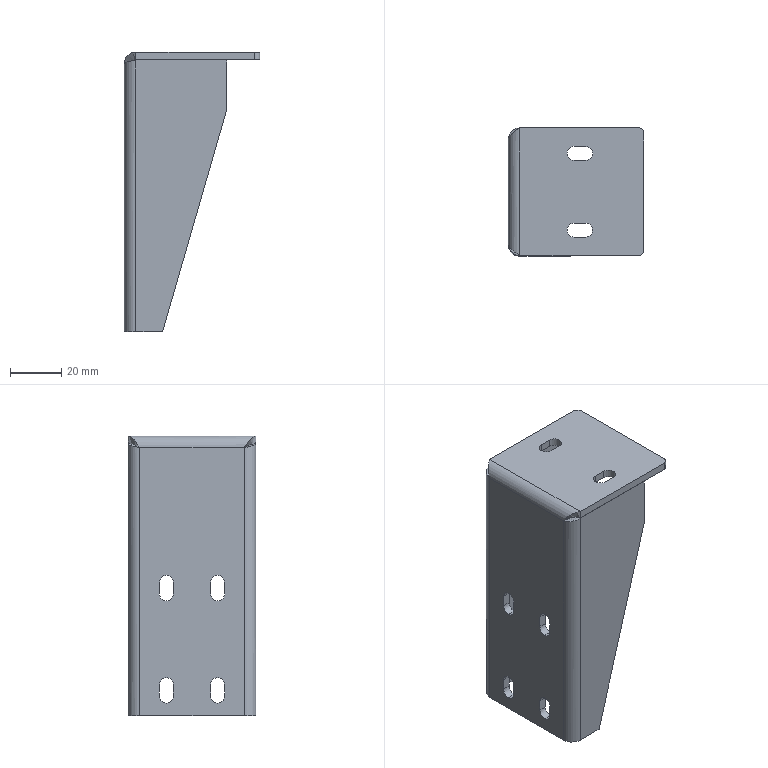Part | STEP file | lower return mounting plate | 1 solid | 62 faces | box 53 x 50 x 109.5 mm | volume 39119 mm3 | plane 34 | cylinder 24 | spline 4 | commonest cylinder face diameters 5.5 x16 3 x3 9 x3 4 x2